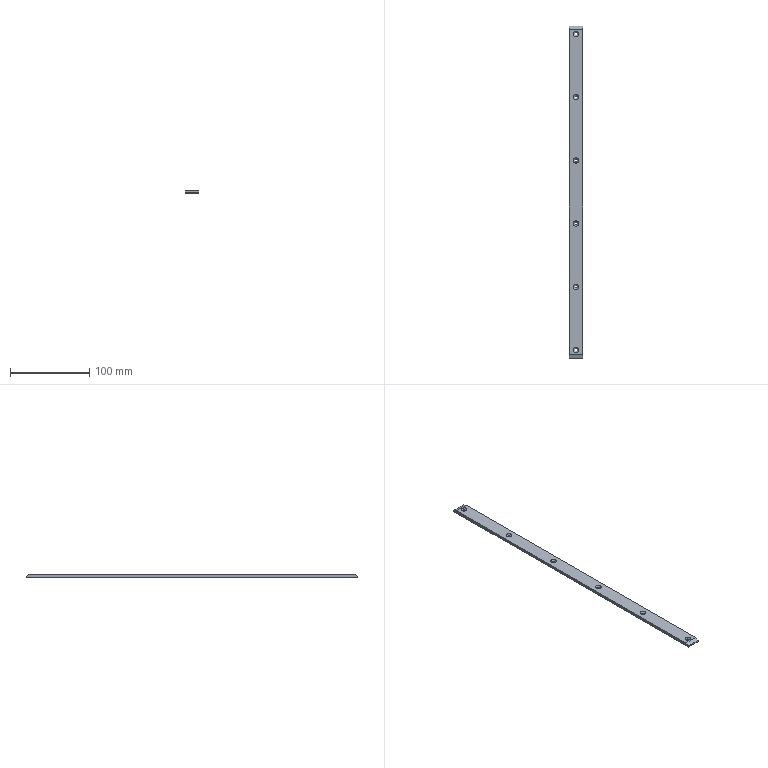Part | NX | features BREP 1 | 1 solid | 32 faces | box 17 x 420 x 4 mm | volume 28032 mm3 | cone 12 | cylinder 12 | plane 8 | commonest cylinder face diameters 3.4 x12
STEP:
#1=CARTESIAN_POINT('',(-8.5,-210.,2.));
#2=VERTEX_POINT('',#1);
#3=CARTESIAN_POINT('',(-8.5,-205.,4.));
#4=VERTEX_POINT('',#3);
#5=CARTESIAN_POINT('',(-8.5,-205.,4.));
#6=DIRECTION('',(0.,0.9285,0.3714));
#7=VECTOR('',#6,1000.);
#8=LINE('',#5,#7);
#9=EDGE_CURVE('',#2,#4,#8,.T.);
#10=ORIENTED_EDGE('',*,*,#9,.F.);
#11=CARTESIAN_POINT('',(8.5,-210.,2.));
#12=VERTEX_POINT('',#11);
#13=CARTESIAN_POINT('',(-8.5,-210.,2.));
#14=DIRECTION('',(-1.,0.,0.));
#15=VECTOR('',#14,1000.);
#16=LINE('',#13,#15);
#17=EDGE_CURVE('',#12,#2,#16,.T.);
#18=ORIENTED_EDGE('',*,*,#17,.F.);
#19=CARTESIAN_POINT('',(8.5,-205.,4.));
#20=VERTEX_POINT('',#19);
#21=CARTESIAN_POINT('',(8.5,-205.,4.));
#22=DIRECTION('',(0.,-0.9285,-0.3714));
#23=VECTOR('',#22,1000.);
#24=LINE('',#21,#23);
#25=EDGE_CURVE('',#20,#12,#24,.T.);
#26=ORIENTED_EDGE('',*,*,#25,.F.);
#27=CARTESIAN_POINT('',(0.,-205.,4.));
#28=DIRECTION('',(1.,0.,0.));
#29=VECTOR('',#28,1000.);
#30=LINE('',#27,#29);
#31=EDGE_CURVE('',#4,#20,#30,.T.);
#32=ORIENTED_EDGE('',*,*,#31,.F.);
#33=EDGE_LOOP('',(#10,#18,#26,#32));
#34=FACE_BOUND('',#33,.T.);
#35=CARTESIAN_POINT('',(0.,-205.,4.));
#36=DIRECTION('',(0.,0.3714,-0.9285));
#37=DIRECTION('',(1.,0.,0.));
#38=AXIS2_PLACEMENT_3D('',#35,#36,#37);
#39=PLANE('',#38);
#40=ADVANCED_FACE('',(#34),#39,.F.);
#41=CARTESIAN_POINT('',(8.5,210.,2.));
#42=VERTEX_POINT('',#41);
#43=CARTESIAN_POINT('',(8.5,205.,4.));
#44=VERTEX_POINT('',#43);
#45=CARTESIAN_POINT('',(8.5,205.,4.));
#46=DIRECTION('',(0.,-0.9285,0.3714));
#47=VECTOR('',#46,1000.);
#48=LINE('',#45,#47);
#49=EDGE_CURVE('',#42,#44,#48,.T.);
#50=ORIENTED_EDGE('',*,*,#49,.F.);
#51=CARTESIAN_POINT('',(-8.5,210.,2.));
#52=VERTEX_POINT('',#51);
#53=CARTESIAN_POINT('',(-8.5,210.,2.));
#54=DIRECTION('',(1.,0.,0.));
#55=VECTOR('',#54,1000.);
#56=LINE('',#53,#55);
#57=EDGE_CURVE('',#52,#42,#56,.T.);
#58=ORIENTED_EDGE('',*,*,#57,.F.);
#59=CARTESIAN_POINT('',(-8.5,205.,4.));
#60=VERTEX_POINT('',#59);
#61=CARTESIAN_POINT('',(-8.5,205.,4.));
#62=DIRECTION('',(0.,0.9285,-0.3714));
#63=VECTOR('',#62,1000.);
#64=LINE('',#61,#63);
#65=EDGE_CURVE('',#60,#52,#64,.T.);
#66=ORIENTED_EDGE('',*,*,#65,.F.);
#67=CARTESIAN_POINT('',(0.,205.,4.));
#68=DIRECTION('',(-1.,0.,0.));
#69=VECTOR('',#68,1000.);
#70=LINE('',#67,#69);
#71=EDGE_CURVE('',#44,#60,#70,.T.);
#72=ORIENTED_EDGE('',*,*,#71,.F.);
#73=EDGE_LOOP('',(#50,#58,#66,#72));
#74=FACE_BOUND('',#73,.T.);
#75=CARTESIAN_POINT('',(0.,205.,4.));
#76=DIRECTION('',(0.,-0.3714,-0.9285));
#77=DIRECTION('',(-1.,0.,0.));
#78=AXIS2_PLACEMENT_3D('',#75,#76,#77);
#79=PLANE('',#78);
#80=ADVANCED_FACE('',(#74),#79,.F.);
#81=CARTESIAN_POINT('',(-3.5,-200.,4.));
#82=VERTEX_POINT('',#81);
#83=CARTESIAN_POINT('',(-1.7,-200.,2.2));
#84=VERTEX_POINT('',#83);
#85=CARTESIAN_POINT('',(-3.5,-200.,4.));
#86=DIRECTION('',(-0.7071,0.,0.7071));
#87=VECTOR('',#86,1000.);
#88=LINE('',#85,#87);
#89=EDGE_CURVE('',#82,#84,#88,.F.);
#90=ORIENTED_EDGE('',*,*,#89,.T.);
#91=CARTESIAN_POINT('',(1.7,-200.,2.2));
#92=VERTEX_POINT('',#91);
#93=CARTESIAN_POINT('',(0.,-200.,2.2));
#94=DIRECTION('',(0.,0.,1.));
#95=DIRECTION('',(1.,0.,0.));
#96=AXIS2_PLACEMENT_3D('',#93,#94,#95);
#97=CIRCLE('',#96,1.7);
#98=EDGE_CURVE('',#92,#84,#97,.T.);
#99=ORIENTED_EDGE('',*,*,#98,.F.);
#100=CARTESIAN_POINT('',(3.5,-200.,4.));
#101=VERTEX_POINT('',#100);
#102=CARTESIAN_POINT('',(3.5,-200.,4.));
#103=DIRECTION('',(0.7071,0.,0.7071));
#104=VECTOR('',#103,1000.);
#105=LINE('',#102,#104);
#106=EDGE_CURVE('',#101,#92,#105,.F.);
#107=ORIENTED_EDGE('',*,*,#106,.F.);
#108=CARTESIAN_POINT('',(0.,-200.,4.));
#109=DIRECTION('',(0.,0.,1.));
#110=DIRECTION('',(1.,0.,0.));
#111=AXIS2_PLACEMENT_3D('',#108,#109,#110);
#112=CIRCLE('',#111,3.5);
#113=EDGE_CURVE('',#101,#82,#112,.T.);
#114=ORIENTED_EDGE('',*,*,#113,.T.);
#115=EDGE_LOOP('',(#90,#99,#107,#114));
#116=FACE_BOUND('',#115,.T.);
#117=CARTESIAN_POINT('',(0.,-200.,4.));
#118=DIRECTION('',(0.,0.,1.));
#119=DIRECTION('',(1.,0.,0.));
#120=AXIS2_PLACEMENT_3D('',#117,#118,#119);
#121=CONICAL_SURFACE('',#120,3.5,0.7854);
#122=ADVANCED_FACE('',(#116),#121,.F.);
#123=CARTESIAN_POINT('',(-1.7,-200.,0.));
#124=VERTEX_POINT('',#123);
#125=CARTESIAN_POINT('',(-1.7,-200.,4.));
#126=DIRECTION('',(0.,0.,1.));
#127=VECTOR('',#126,1000.);
#128=LINE('',#125,#127);
#129=EDGE_CURVE('',#84,#124,#128,.F.);
#130=ORIENTED_EDGE('',*,*,#129,.T.);
#131=CARTESIAN_POINT('',(1.7,-200.,0.));
#132=VERTEX_POINT('',#131);
#133=CARTESIAN_POINT('',(0.,-200.,0.));
#134=DIRECTION('',(0.,0.,-1.));
#135=DIRECTION('',(-1.,0.,0.));
#136=AXIS2_PLACEMENT_3D('',#133,#134,#135);
#137=CIRCLE('',#136,1.7);
#138=EDGE_CURVE('',#124,#132,#137,.T.);
#139=ORIENTED_EDGE('',*,*,#138,.T.);
#140=CARTESIAN_POINT('',(1.7,-200.,4.));
#141=DIRECTION('',(0.,0.,1.));
#142=VECTOR('',#141,1000.);
#143=LINE('',#140,#142);
#144=EDGE_CURVE('',#92,#132,#143,.F.);
#145=ORIENTED_EDGE('',*,*,#144,.F.);
#146=ORIENTED_EDGE('',*,*,#98,.T.);
#147=EDGE_LOOP('',(#130,#139,#145,#146));
#148=FACE_BOUND('',#147,.T.);
#149=CARTESIAN_POINT('',(0.,-200.,4.));
#150=DIRECTION('',(0.,0.,1.));
#151=DIRECTION('',(1.,0.,0.));
#152=AXIS2_PLACEMENT_3D('',#149,#150,#151);
#153=CYLINDRICAL_SURFACE('',#152,1.7);
#154=ADVANCED_FACE('',(#148),#153,.F.);
#155=CARTESIAN_POINT('',(-3.5,-120.,4.));
#156=VERTEX_POINT('',#155);
#157=CARTESIAN_POINT('',(-1.7,-120.,2.2));
#158=VERTEX_POINT('',#157);
#159=CARTESIAN_POINT('',(-3.5,-120.,4.));
#160=DIRECTION('',(-0.7071,0.,0.7071));
#161=VECTOR('',#160,1000.);
#162=LINE('',#159,#161);
#163=EDGE_CURVE('',#156,#158,#162,.F.);
#164=ORIENTED_EDGE('',*,*,#163,.T.);
#165=CARTESIAN_POINT('',(1.7,-120.,2.2));
#166=VERTEX_POINT('',#165);
#167=CARTESIAN_POINT('',(0.,-120.,2.2));
#168=DIRECTION('',(0.,0.,1.));
#169=DIRECTION('',(1.,0.,0.));
#170=AXIS2_PLACEMENT_3D('',#167,#168,#169);
#171=CIRCLE('',#170,1.7);
#172=EDGE_CURVE('',#166,#158,#171,.T.);
#173=ORIENTED_EDGE('',*,*,#172,.F.);
#174=CARTESIAN_POINT('',(3.5,-120.,4.));
#175=VERTEX_POINT('',#174);
#176=CARTESIAN_POINT('',(3.5,-120.,4.));
#177=DIRECTION('',(0.7071,0.,0.7071));
#178=VECTOR('',#177,1000.);
#179=LINE('',#176,#178);
#180=EDGE_CURVE('',#175,#166,#179,.F.);
#181=ORIENTED_EDGE('',*,*,#180,.F.);
#182=CARTESIAN_POINT('',(0.,-120.,4.));
#183=DIRECTION('',(0.,0.,1.));
#184=DIRECTION('',(1.,0.,0.));
#185=AXIS2_PLACEMENT_3D('',#182,#183,#184);
#186=CIRCLE('',#185,3.5);
#187=EDGE_CURVE('',#175,#156,#186,.T.);
#188=ORIENTED_EDGE('',*,*,#187,.T.);
#189=EDGE_LOOP('',(#164,#173,#181,#188));
#190=FACE_BOUND('',#189,.T.);
#191=CARTESIAN_POINT('',(0.,-120.,4.));
#192=DIRECTION('',(0.,0.,1.));
#193=DIRECTION('',(1.,0.,0.));
#194=AXIS2_PLACEMENT_3D('',#191,#192,#193);
#195=CONICAL_SURFACE('',#194,3.5,0.7854);
#196=ADVANCED_FACE('',(#190),#195,.F.);
#197=CARTESIAN_POINT('',(-1.7,-120.,0.));
#198=VERTEX_POINT('',#197);
#199=CARTESIAN_POINT('',(-1.7,-120.,4.));
#200=DIRECTION('',(0.,0.,1.));
#201=VECTOR('',#200,1000.);
#202=LINE('',#199,#201);
#203=EDGE_CURVE('',#158,#198,#202,.F.);
#204=ORIENTED_EDGE('',*,*,#203,.T.);
#205=CARTESIAN_POINT('',(1.7,-120.,0.));
#206=VERTEX_POINT('',#205);
#207=CARTESIAN_POINT('',(0.,-120.,0.));
#208=DIRECTION('',(0.,0.,-1.));
#209=DIRECTION('',(-1.,0.,0.));
#210=AXIS2_PLACEMENT_3D('',#207,#208,#209);
#211=CIRCLE('',#210,1.7);
#212=EDGE_CURVE('',#198,#206,#211,.T.);
#213=ORIENTED_EDGE('',*,*,#212,.T.);
#214=CARTESIAN_POINT('',(1.7,-120.,4.));
#215=DIRECTION('',(0.,0.,1.));
#216=VECTOR('',#215,1000.);
#217=LINE('',#214,#216);
#218=EDGE_CURVE('',#166,#206,#217,.F.);
#219=ORIENTED_EDGE('',*,*,#218,.F.);
#220=ORIENTED_EDGE('',*,*,#172,.T.);
#221=EDGE_LOOP('',(#204,#213,#219,#220));
#222=FACE_BOUND('',#221,.T.);
#223=CARTESIAN_POINT('',(0.,-120.,4.));
#224=DIRECTION('',(0.,0.,1.));
#225=DIRECTION('',(1.,0.,0.));
#226=AXIS2_PLACEMENT_3D('',#223,#224,#225);
#227=CYLINDRICAL_SURFACE('',#226,1.7);
#228=ADVANCED_FACE('',(#222),#227,.F.);
#229=CARTESIAN_POINT('',(-3.5,-40.,4.));
#230=VERTEX_POINT('',#229);
#231=CARTESIAN_POINT('',(-1.7,-40.,2.2));
#232=VERTEX_POINT('',#231);
#233=CARTESIAN_POINT('',(-3.5,-40.,4.));
#234=DIRECTION('',(-0.7071,0.,0.7071));
#235=VECTOR('',#234,1000.);
#236=LINE('',#233,#235);
#237=EDGE_CURVE('',#230,#232,#236,.F.);
#238=ORIENTED_EDGE('',*,*,#237,.T.);
#239=CARTESIAN_POINT('',(1.7,-40.,2.2));
#240=VERTEX_POINT('',#239);
#241=CARTESIAN_POINT('',(0.,-40.,2.2));
#242=DIRECTION('',(0.,0.,1.));
#243=DIRECTION('',(1.,0.,0.));
#244=AXIS2_PLACEMENT_3D('',#241,#242,#243);
#245=CIRCLE('',#244,1.7);
#246=EDGE_CURVE('',#240,#232,#245,.T.);
#247=ORIENTED_EDGE('',*,*,#246,.F.);
#248=CARTESIAN_POINT('',(3.5,-40.,4.));
#249=VERTEX_POINT('',#248);
#250=CARTESIAN_POINT('',(3.5,-40.,4.));
#251=DIRECTION('',(0.7071,0.,0.7071));
#252=VECTOR('',#251,1000.);
#253=LINE('',#250,#252);
#254=EDGE_CURVE('',#249,#240,#253,.F.);
#255=ORIENTED_EDGE('',*,*,#254,.F.);
#256=CARTESIAN_POINT('',(0.,-40.,4.));
#257=DIRECTION('',(0.,0.,1.));
#258=DIRECTION('',(1.,0.,0.));
#259=AXIS2_PLACEMENT_3D('',#256,#257,#258);
#260=CIRCLE('',#259,3.5);
#261=EDGE_CURVE('',#249,#230,#260,.T.);
#262=ORIENTED_EDGE('',*,*,#261,.T.);
#263=EDGE_LOOP('',(#238,#247,#255,#262));
#264=FACE_BOUND('',#263,.T.);
#265=CARTESIAN_POINT('',(0.,-40.,4.));
#266=DIRECTION('',(0.,0.,1.));
#267=DIRECTION('',(1.,0.,0.));
#268=AXIS2_PLACEMENT_3D('',#265,#266,#267);
#269=CONICAL_SURFACE('',#268,3.5,0.7854);
#270=ADVANCED_FACE('',(#264),#269,.F.);
#271=CARTESIAN_POINT('',(-1.7,-40.,0.));
#272=VERTEX_POINT('',#271);
#273=CARTESIAN_POINT('',(-1.7,-40.,4.));
#274=DIRECTION('',(0.,0.,1.));
#275=VECTOR('',#274,1000.);
#276=LINE('',#273,#275);
#277=EDGE_CURVE('',#232,#272,#276,.F.);
#278=ORIENTED_EDGE('',*,*,#277,.T.);
#279=CARTESIAN_POINT('',(1.7,-40.,0.));
#280=VERTEX_POINT('',#279);
#281=CARTESIAN_POINT('',(0.,-40.,0.));
#282=DIRECTION('',(0.,0.,-1.));
#283=DIRECTION('',(-1.,0.,0.));
#284=AXIS2_PLACEMENT_3D('',#281,#282,#283);
#285=CIRCLE('',#284,1.7);
#286=EDGE_CURVE('',#272,#280,#285,.T.);
#287=ORIENTED_EDGE('',*,*,#286,.T.);
#288=CARTESIAN_POINT('',(1.7,-40.,4.));
#289=DIRECTION('',(0.,0.,1.));
#290=VECTOR('',#289,1000.);
#291=LINE('',#288,#290);
#292=EDGE_CURVE('',#240,#280,#291,.F.);
#293=ORIENTED_EDGE('',*,*,#292,.F.);
#294=ORIENTED_EDGE('',*,*,#246,.T.);
#295=EDGE_LOOP('',(#278,#287,#293,#294));
#296=FACE_BOUND('',#295,.T.);
#297=CARTESIAN_POINT('',(0.,-40.,4.));
#298=DIRECTION('',(0.,0.,1.));
#299=DIRECTION('',(1.,0.,0.));
#300=AXIS2_PLACEMENT_3D('',#297,#298,#299);
#301=CYLINDRICAL_SURFACE('',#300,1.7);
#302=ADVANCED_FACE('',(#296),#301,.F.);
#303=CARTESIAN_POINT('',(-3.5,40.,4.));
#304=VERTEX_POINT('',#303);
#305=CARTESIAN_POINT('',(-1.7,40.,2.2));
#306=VERTEX_POINT('',#305);
#307=CARTESIAN_POINT('',(-3.5,40.,4.));
#308=DIRECTION('',(-0.7071,0.,0.7071));
#309=VECTOR('',#308,1000.);
#310=LINE('',#307,#309);
#311=EDGE_CURVE('',#304,#306,#310,.F.);
#312=ORIENTED_EDGE('',*,*,#311,.T.);
#313=CARTESIAN_POINT('',(1.7,40.,2.2));
#314=VERTEX_POINT('',#313);
#315=CARTESIAN_POINT('',(0.,40.,2.2));
#316=DIRECTION('',(0.,0.,1.));
#317=DIRECTION('',(1.,0.,0.));
#318=AXIS2_PLACEMENT_3D('',#315,#316,#317);
#319=CIRCLE('',#318,1.7);
#320=EDGE_CURVE('',#314,#306,#319,.T.);
#321=ORIENTED_EDGE('',*,*,#320,.F.);
#322=CARTESIAN_POINT('',(3.5,40.,4.));
#323=VERTEX_POINT('',#322);
#324=CARTESIAN_POINT('',(3.5,40.,4.));
#325=DIRECTION('',(0.7071,0.,0.7071));
#326=VECTOR('',#325,1000.);
#327=LINE('',#324,#326);
#328=EDGE_CURVE('',#323,#314,#327,.F.);
#329=ORIENTED_EDGE('',*,*,#328,.F.);
#330=CARTESIAN_POINT('',(0.,40.,4.));
#331=DIRECTION('',(0.,0.,1.));
#332=DIRECTION('',(1.,0.,0.));
#333=AXIS2_PLACEMENT_3D('',#330,#331,#332);
#334=CIRCLE('',#333,3.5);
#335=EDGE_CURVE('',#323,#304,#334,.T.);
#336=ORIENTED_EDGE('',*,*,#335,.T.);
#337=EDGE_LOOP('',(#312,#321,#329,#336));
#338=FACE_BOUND('',#337,.T.);
#339=CARTESIAN_POINT('',(0.,40.,4.));
#340=DIRECTION('',(0.,0.,1.));
#341=DIRECTION('',(1.,0.,0.));
#342=AXIS2_PLACEMENT_3D('',#339,#340,#341);
#343=CONICAL_SURFACE('',#342,3.5,0.7854);
#344=ADVANCED_FACE('',(#338),#343,.F.);
#345=CARTESIAN_POINT('',(-1.7,40.,0.));
#346=VERTEX_POINT('',#345);
#347=CARTESIAN_POINT('',(-1.7,40.,4.));
#348=DIRECTION('',(0.,0.,1.));
#349=VECTOR('',#348,1000.);
#350=LINE('',#347,#349);
#351=EDGE_CURVE('',#306,#346,#350,.F.);
#352=ORIENTED_EDGE('',*,*,#351,.T.);
#353=CARTESIAN_POINT('',(1.7,40.,0.));
#354=VERTEX_POINT('',#353);
#355=CARTESIAN_POINT('',(0.,40.,0.));
#356=DIRECTION('',(0.,0.,-1.));
#357=DIRECTION('',(-1.,0.,0.));
#358=AXIS2_PLACEMENT_3D('',#355,#356,#357);
#359=CIRCLE('',#358,1.7);
#360=EDGE_CURVE('',#346,#354,#359,.T.);
#361=ORIENTED_EDGE('',*,*,#360,.T.);
#362=CARTESIAN_POINT('',(1.7,40.,4.));
#363=DIRECTION('',(0.,0.,1.));
#364=VECTOR('',#363,1000.);
#365=LINE('',#362,#364);
#366=EDGE_CURVE('',#314,#354,#365,.F.);
#367=ORIENTED_EDGE('',*,*,#366,.F.);
#368=ORIENTED_EDGE('',*,*,#320,.T.);
#369=EDGE_LOOP('',(#352,#361,#367,#368));
#370=FACE_BOUND('',#369,.T.);
#371=CARTESIAN_POINT('',(0.,40.,4.));
#372=DIRECTION('',(0.,0.,1.));
#373=DIRECTION('',(1.,0.,0.));
#374=AXIS2_PLACEMENT_3D('',#371,#372,#373);
#375=CYLINDRICAL_SURFACE('',#374,1.7);
#376=ADVANCED_FACE('',(#370),#375,.F.);
#377=CARTESIAN_POINT('',(-3.5,120.,4.));
#378=VERTEX_POINT('',#377);
#379=CARTESIAN_POINT('',(-1.7,120.,2.2));
#380=VERTEX_POINT('',#379);
#381=CARTESIAN_POINT('',(-3.5,120.,4.));
#382=DIRECTION('',(-0.7071,0.,0.7071));
#383=VECTOR('',#382,1000.);
#384=LINE('',#381,#383);
#385=EDGE_CURVE('',#378,#380,#384,.F.);
#386=ORIENTED_EDGE('',*,*,#385,.T.);
#387=CARTESIAN_POINT('',(1.7,120.,2.2));
#388=VERTEX_POINT('',#387);
#389=CARTESIAN_POINT('',(0.,120.,2.2));
#390=DIRECTION('',(0.,0.,1.));
#391=DIRECTION('',(1.,0.,0.));
#392=AXIS2_PLACEMENT_3D('',#389,#390,#391);
#393=CIRCLE('',#392,1.7);
#394=EDGE_CURVE('',#388,#380,#393,.T.);
#395=ORIENTED_EDGE('',*,*,#394,.F.);
#396=CARTESIAN_POINT('',(3.5,120.,4.));
#397=VERTEX_POINT('',#396);
#398=CARTESIAN_POINT('',(3.5,120.,4.));
#399=DIRECTION('',(0.7071,0.,0.7071));
#400=VECTOR('',#399,1000.);
#401=LINE('',#398,#400);
#402=EDGE_CURVE('',#397,#388,#401,.F.);
#403=ORIENTED_EDGE('',*,*,#402,.F.);
#404=CARTESIAN_POINT('',(0.,120.,4.));
#405=DIRECTION('',(0.,0.,1.));
#406=DIRECTION('',(1.,0.,0.));
#407=AXIS2_PLACEMENT_3D('',#404,#405,#406);
#408=CIRCLE('',#407,3.5);
#409=EDGE_CURVE('',#397,#378,#408,.T.);
#410=ORIENTED_EDGE('',*,*,#409,.T.);
#411=EDGE_LOOP('',(#386,#395,#403,#410));
#412=FACE_BOUND('',#411,.T.);
#413=CARTESIAN_POINT('',(0.,120.,4.));
#414=DIRECTION('',(0.,0.,1.));
#415=DIRECTION('',(1.,0.,0.));
#416=AXIS2_PLACEMENT_3D('',#413,#414,#415);
#417=CONICAL_SURFACE('',#416,3.5,0.7854);
#418=ADVANCED_FACE('',(#412),#417,.F.);
#419=CARTESIAN_POINT('',(-1.7,120.,0.));
#420=VERTEX_POINT('',#419);
#421=CARTESIAN_POINT('',(-1.7,120.,4.));
#422=DIRECTION('',(0.,0.,1.));
#423=VECTOR('',#422,1000.);
#424=LINE('',#421,#423);
#425=EDGE_CURVE('',#380,#420,#424,.F.);
#426=ORIENTED_EDGE('',*,*,#425,.T.);
#427=CARTESIAN_POINT('',(1.7,120.,0.));
#428=VERTEX_POINT('',#427);
#429=CARTESIAN_POINT('',(0.,120.,0.));
#430=DIRECTION('',(0.,0.,-1.));
#431=DIRECTION('',(-1.,0.,0.));
#432=AXIS2_PLACEMENT_3D('',#429,#430,#431);
#433=CIRCLE('',#432,1.7);
#434=EDGE_CURVE('',#420,#428,#433,.T.);
#435=ORIENTED_EDGE('',*,*,#434,.T.);
#436=CARTESIAN_POINT('',(1.7,120.,4.));
#437=DIRECTION('',(0.,0.,1.));
#438=VECTOR('',#437,1000.);
#439=LINE('',#436,#438);
#440=EDGE_CURVE('',#388,#428,#439,.F.);
#441=ORIENTED_EDGE('',*,*,#440,.F.);
#442=ORIENTED_EDGE('',*,*,#394,.T.);
#443=EDGE_LOOP('',(#426,#435,#441,#442));
#444=FACE_BOUND('',#443,.T.);
#445=CARTESIAN_POINT('',(0.,120.,4.));
#446=DIRECTION('',(0.,0.,1.));
#447=DIRECTION('',(1.,0.,0.));
#448=AXIS2_PLACEMENT_3D('',#445,#446,#447);
#449=CYLINDRICAL_SURFACE('',#448,1.7);
#450=ADVANCED_FACE('',(#444),#449,.F.);
#451=CARTESIAN_POINT('',(-3.5,200.,4.));
#452=VERTEX_POINT('',#451);
#453=CARTESIAN_POINT('',(-1.7,200.,2.2));
#454=VERTEX_POINT('',#453);
#455=CARTESIAN_POINT('',(-3.5,200.,4.));
#456=DIRECTION('',(-0.7071,0.,0.7071));
#457=VECTOR('',#456,1000.);
#458=LINE('',#455,#457);
#459=EDGE_CURVE('',#452,#454,#458,.F.);
#460=ORIENTED_EDGE('',*,*,#459,.T.);
#461=CARTESIAN_POINT('',(1.7,200.,2.2));
#462=VERTEX_POINT('',#461);
#463=CARTESIAN_POINT('',(0.,200.,2.2));
#464=DIRECTION('',(0.,0.,1.));
#465=DIRECTION('',(1.,0.,0.));
#466=AXIS2_PLACEMENT_3D('',#463,#464,#465);
#467=CIRCLE('',#466,1.7);
#468=EDGE_CURVE('',#462,#454,#467,.T.);
#469=ORIENTED_EDGE('',*,*,#468,.F.);
#470=CARTESIAN_POINT('',(3.5,200.,4.));
#471=VERTEX_POINT('',#470);
#472=CARTESIAN_POINT('',(3.5,200.,4.));
#473=DIRECTION('',(0.7071,0.,0.7071));
#474=VECTOR('',#473,1000.);
#475=LINE('',#472,#474);
#476=EDGE_CURVE('',#471,#462,#475,.F.);
#477=ORIENTED_EDGE('',*,*,#476,.F.);
#478=CARTESIAN_POINT('',(0.,200.,4.));
#479=DIRECTION('',(0.,0.,1.));
#480=DIRECTION('',(1.,0.,0.));
#481=AXIS2_PLACEMENT_3D('',#478,#479,#480);
#482=CIRCLE('',#481,3.5);
#483=EDGE_CURVE('',#471,#452,#482,.T.);
#484=ORIENTED_EDGE('',*,*,#483,.T.);
#485=EDGE_LOOP('',(#460,#469,#477,#484));
#486=FACE_BOUND('',#485,.T.);
#487=CARTESIAN_POINT('',(0.,200.,4.));
#488=DIRECTION('',(0.,0.,1.));
#489=DIRECTION('',(1.,0.,0.));
#490=AXIS2_PLACEMENT_3D('',#487,#488,#489);
#491=CONICAL_SURFACE('',#490,3.5,0.7854);
#492=ADVANCED_FACE('',(#486),#491,.F.);
#493=CARTESIAN_POINT('',(-1.7,200.,0.));
#494=VERTEX_POINT('',#493);
#495=CARTESIAN_POINT('',(-1.7,200.,4.));
#496=DIRECTION('',(0.,0.,1.));
#497=VECTOR('',#496,1000.);
#498=LINE('',#495,#497);
#499=EDGE_CURVE('',#454,#494,#498,.F.);
#500=ORIENTED_EDGE('',*,*,#499,.T.);
#501=CARTESIAN_POINT('',(1.7,200.,0.));
#502=VERTEX_POINT('',#501);
#503=CARTESIAN_POINT('',(0.,200.,0.));
#504=DIRECTION('',(0.,0.,-1.));
#505=DIRECTION('',(-1.,0.,0.));
#506=AXIS2_PLACEMENT_3D('',#503,#504,#505);
#507=CIRCLE('',#506,1.7);
#508=EDGE_CURVE('',#494,#502,#507,.T.);
#509=ORIENTED_EDGE('',*,*,#508,.T.);
#510=CARTESIAN_POINT('',(1.7,200.,4.));
#511=DIRECTION('',(0.,0.,1.));
#512=VECTOR('',#511,1000.);
#513=LINE('',#510,#512);
#514=EDGE_CURVE('',#462,#502,#513,.F.);
#515=ORIENTED_EDGE('',*,*,#514,.F.);
#516=ORIENTED_EDGE('',*,*,#468,.T.);
#517=EDGE_LOOP('',(#500,#509,#515,#516));
#518=FACE_BOUND('',#517,.T.);
#519=CARTESIAN_POINT('',(0.,200.,4.));
#520=DIRECTION('',(0.,0.,1.));
#521=DIRECTION('',(1.,0.,0.));
#522=AXIS2_PLACEMENT_3D('',#519,#520,#521);
#523=CYLINDRICAL_SURFACE('',#522,1.7);
#524=ADVANCED_FACE('',(#518),#523,.F.);
#525=CARTESIAN_POINT('',(8.5,-210.,0.));
#526=VERTEX_POINT('',#525);
#527=CARTESIAN_POINT('',(8.5,210.,0.));
#528=VERTEX_POINT('',#527);
#529=CARTESIAN_POINT('',(8.5,-210.,0.));
#530=DIRECTION('',(0.,1.,0.));
#531=VECTOR('',#530,1000.);
#532=LINE('',#529,#531);
#533=EDGE_CURVE('',#526,#528,#532,.T.);
#534=ORIENTED_EDGE('',*,*,#533,.F.);
#535=CARTESIAN_POINT('',(-8.5,-210.,0.));
#536=VERTEX_POINT('',#535);
#537=CARTESIAN_POINT('',(-8.5,-210.,0.));
#538=DIRECTION('',(1.,0.,0.));
#539=VECTOR('',#538,1000.);
#540=LINE('',#537,#539);
#541=EDGE_CURVE('',#536,#526,#540,.T.);
#542=ORIENTED_EDGE('',*,*,#541,.F.);
#543=CARTESIAN_POINT('',(-8.5,210.,0.));
#544=VERTEX_POINT('',#543);
#545=CARTESIAN_POINT('',(-8.5,-210.,0.));
#546=DIRECTION('',(0.,-1.,0.));
#547=VECTOR('',#546,1000.);
#548=LINE('',#545,#547);
#549=EDGE_CURVE('',#544,#536,#548,.T.);
#550=ORIENTED_EDGE('',*,*,#549,.F.);
#551=CARTESIAN_POINT('',(-8.5,210.,0.));
#552=DIRECTION('',(-1.,0.,0.));
#553=VECTOR('',#552,1000.);
#554=LINE('',#551,#553);
#555=EDGE_CURVE('',#528,#544,#554,.T.);
#556=ORIENTED_EDGE('',*,*,#555,.F.);
#557=EDGE_LOOP('',(#534,#542,#550,#556));
#558=FACE_BOUND('',#557,.T.);
#559=CARTESIAN_POINT('',(0.,200.,0.));
#560=DIRECTION('',(0.,0.,-1.));
#561=DIRECTION('',(-1.,0.,0.));
#562=AXIS2_PLACEMENT_3D('',#559,#560,#561);
#563=CIRCLE('',#562,1.7);
#564=EDGE_CURVE('',#502,#494,#563,.T.);
#565=ORIENTED_EDGE('',*,*,#564,.F.);
#566=ORIENTED_EDGE('',*,*,#508,.F.);
#567=EDGE_LOOP('',(#565,#566));
#568=FACE_BOUND('',#567,.T.);
#569=CARTESIAN_POINT('',(0.,120.,0.));
#570=DIRECTION('',(0.,0.,-1.));
#571=DIRECTION('',(-1.,0.,0.));
#572=AXIS2_PLACEMENT_3D('',#569,#570,#571);
#573=CIRCLE('',#572,1.7);
#574=EDGE_CURVE('',#428,#420,#573,.T.);
#575=ORIENTED_EDGE('',*,*,#574,.F.);
#576=ORIENTED_EDGE('',*,*,#434,.F.);
#577=EDGE_LOOP('',(#575,#576));
#578=FACE_BOUND('',#577,.T.);
#579=CARTESIAN_POINT('',(0.,40.,0.));
#580=DIRECTION('',(0.,0.,-1.));
#581=DIRECTION('',(-1.,0.,0.));
#582=AXIS2_PLACEMENT_3D('',#579,#580,#581);
#583=CIRCLE('',#582,1.7);
#584=EDGE_CURVE('',#354,#346,#583,.T.);
#585=ORIENTED_EDGE('',*,*,#584,.F.);
#586=ORIENTED_EDGE('',*,*,#360,.F.);
#587=EDGE_LOOP('',(#585,#586));
#588=FACE_BOUND('',#587,.T.);
#589=CARTESIAN_POINT('',(0.,-40.,0.));
#590=DIRECTION('',(0.,0.,-1.));
#591=DIRECTION('',(-1.,0.,0.));
#592=AXIS2_PLACEMENT_3D('',#589,#590,#591);
#593=CIRCLE('',#592,1.7);
#594=EDGE_CURVE('',#280,#272,#593,.T.);
#595=ORIENTED_EDGE('',*,*,#594,.F.);
#596=ORIENTED_EDGE('',*,*,#286,.F.);
#597=EDGE_LOOP('',(#595,#596));
#598=FACE_BOUND('',#597,.T.);
#599=CARTESIAN_POINT('',(0.,-120.,0.));
#600=DIRECTION('',(0.,0.,-1.));
#601=DIRECTION('',(-1.,0.,0.));
#602=AXIS2_PLACEMENT_3D('',#599,#600,#601);
#603=CIRCLE('',#602,1.7);
#604=EDGE_CURVE('',#206,#198,#603,.T.);
#605=ORIENTED_EDGE('',*,*,#604,.F.);
#606=ORIENTED_EDGE('',*,*,#212,.F.);
#607=EDGE_LOOP('',(#605,#606));
#608=FACE_BOUND('',#607,.T.);
#609=CARTESIAN_POINT('',(0.,-200.,0.));
#610=DIRECTION('',(0.,0.,-1.));
#611=DIRECTION('',(-1.,0.,0.));
#612=AXIS2_PLACEMENT_3D('',#609,#610,#611);
#613=CIRCLE('',#612,1.7);
#614=EDGE_CURVE('',#132,#124,#613,.T.);
#615=ORIENTED_EDGE('',*,*,#614,.F.);
#616=ORIENTED_EDGE('',*,*,#138,.F.);
#617=EDGE_LOOP('',(#615,#616));
#618=FACE_BOUND('',#617,.T.);
#619=CARTESIAN_POINT('',(0.,0.,0.));
#620=DIRECTION('',(0.,0.,-1.));
#621=DIRECTION('',(-1.,0.,0.));
#622=AXIS2_PLACEMENT_3D('',#619,#620,#621);
#623=PLANE('',#622);
#624=ADVANCED_FACE('',(#558,#568,#578,#588,#598,#608,#618),#623,.T.);
#625=CARTESIAN_POINT('',(8.5,-210.,4.));
#626=DIRECTION('',(0.,0.,-1.));
#627=VECTOR('',#626,1000.);
#628=LINE('',#625,#627);
#629=EDGE_CURVE('',#12,#526,#628,.T.);
#630=ORIENTED_EDGE('',*,*,#629,.F.);
#631=ORIENTED_EDGE('',*,*,#17,.T.);
#632=CARTESIAN_POINT('',(-8.5,-210.,4.));
#633=DIRECTION('',(0.,0.,-1.));
#634=VECTOR('',#633,1000.);
#635=LINE('',#632,#634);
#636=EDGE_CURVE('',#2,#536,#635,.T.);
#637=ORIENTED_EDGE('',*,*,#636,.T.);
#638=ORIENTED_EDGE('',*,*,#541,.T.);
#639=EDGE_LOOP('',(#630,#631,#637,#638));
#640=FACE_BOUND('',#639,.T.);
#641=CARTESIAN_POINT('',(-8.5,-210.,4.));
#642=DIRECTION('',(0.,1.,0.));
#643=DIRECTION('',(0.,0.,1.));
#644=AXIS2_PLACEMENT_3D('',#641,#642,#643);
#645=PLANE('',#644);
#646=ADVANCED_FACE('',(#640),#645,.F.);
#647=ORIENTED_EDGE('',*,*,#636,.F.);
#648=ORIENTED_EDGE('',*,*,#9,.T.);
#649=CARTESIAN_POINT('',(-8.5,-210.,4.));
#650=DIRECTION('',(0.,-1.,0.));
#651=VECTOR('',#650,1000.);
#652=LINE('',#649,#651);
#653=EDGE_CURVE('',#60,#4,#652,.T.);
#654=ORIENTED_EDGE('',*,*,#653,.F.);
#655=ORIENTED_EDGE('',*,*,#65,.T.);
#656=CARTESIAN_POINT('',(-8.5,210.,4.));
#657=DIRECTION('',(0.,0.,-1.));
#658=VECTOR('',#657,1000.);
#659=LINE('',#656,#658);
#660=EDGE_CURVE('',#52,#544,#659,.T.);
#661=ORIENTED_EDGE('',*,*,#660,.T.);
#662=ORIENTED_EDGE('',*,*,#549,.T.);
#663=EDGE_LOOP('',(#647,#648,#654,#655,#661,#662));
#664=FACE_BOUND('',#663,.T.);
#665=CARTESIAN_POINT('',(-8.5,-210.,4.));
#666=DIRECTION('',(1.,0.,0.));
#667=DIRECTION('',(0.,0.,-1.));
#668=AXIS2_PLACEMENT_3D('',#665,#666,#667);
#669=PLANE('',#668);
#670=ADVANCED_FACE('',(#664),#669,.F.);
#671=ORIENTED_EDGE('',*,*,#660,.F.);
#672=ORIENTED_EDGE('',*,*,#57,.T.);
#673=CARTESIAN_POINT('',(8.5,210.,4.));
#674=DIRECTION('',(0.,0.,-1.));
#675=VECTOR('',#674,1000.);
#676=LINE('',#673,#675);
#677=EDGE_CURVE('',#42,#528,#676,.T.);
#678=ORIENTED_EDGE('',*,*,#677,.T.);
#679=ORIENTED_EDGE('',*,*,#555,.T.);
#680=EDGE_LOOP('',(#671,#672,#678,#679));
#681=FACE_BOUND('',#680,.T.);
#682=CARTESIAN_POINT('',(-8.5,210.,4.));
#683=DIRECTION('',(0.,-1.,0.));
#684=DIRECTION('',(0.,0.,-1.));
#685=AXIS2_PLACEMENT_3D('',#682,#683,#684);
#686=PLANE('',#685);
#687=ADVANCED_FACE('',(#681),#686,.F.);
#688=CARTESIAN_POINT('',(8.5,-210.,4.));
#689=DIRECTION('',(0.,1.,0.));
#690=VECTOR('',#689,1000.);
#691=LINE('',#688,#690);
#692=EDGE_CURVE('',#20,#44,#691,.T.);
#693=ORIENTED_EDGE('',*,*,#692,.F.);
#694=ORIENTED_EDGE('',*,*,#25,.T.);
#695=ORIENTED_EDGE('',*,*,#629,.T.);
#696=ORIENTED_EDGE('',*,*,#533,.T.);
#697=ORIENTED_EDGE('',*,*,#677,.F.);
#698=ORIENTED_EDGE('',*,*,#49,.T.);
#699=EDGE_LOOP('',(#693,#694,#695,#696,#697,#698));
#700=FACE_BOUND('',#699,.T.);
#701=CARTESIAN_POINT('',(8.5,-210.,4.));
#702=DIRECTION('',(-1.,0.,0.));
#703=DIRECTION('',(0.,0.,1.));
#704=AXIS2_PLACEMENT_3D('',#701,#702,#703);
#705=PLANE('',#704);
#706=ADVANCED_FACE('',(#700),#705,.F.);
#707=ORIENTED_EDGE('',*,*,#261,.F.);
#708=CARTESIAN_POINT('',(0.,-40.,4.));
#709=DIRECTION('',(0.,0.,1.));
#710=DIRECTION('',(1.,0.,0.));
#711=AXIS2_PLACEMENT_3D('',#708,#709,#710);
#712=CIRCLE('',#711,3.5);
#713=EDGE_CURVE('',#230,#249,#712,.T.);
#714=ORIENTED_EDGE('',*,*,#713,.F.);
#715=EDGE_LOOP('',(#707,#714));
#716=FACE_BOUND('',#715,.T.);
#717=ORIENTED_EDGE('',*,*,#653,.T.);
#718=ORIENTED_EDGE('',*,*,#31,.T.);
#719=ORIENTED_EDGE('',*,*,#692,.T.);
#720=ORIENTED_EDGE('',*,*,#71,.T.);
#721=EDGE_LOOP('',(#717,#718,#719,#720));
#722=FACE_BOUND('',#721,.T.);
#723=ORIENTED_EDGE('',*,*,#483,.F.);
#724=CARTESIAN_POINT('',(0.,200.,4.));
#725=DIRECTION('',(0.,0.,1.));
#726=DIRECTION('',(1.,0.,0.));
#727=AXIS2_PLACEMENT_3D('',#724,#725,#726);
#728=CIRCLE('',#727,3.5);
#729=EDGE_CURVE('',#452,#471,#728,.T.);
#730=ORIENTED_EDGE('',*,*,#729,.F.);
#731=EDGE_LOOP('',(#723,#730));
#732=FACE_BOUND('',#731,.T.);
#733=ORIENTED_EDGE('',*,*,#409,.F.);
#734=CARTESIAN_POINT('',(0.,120.,4.));
#735=DIRECTION('',(0.,0.,1.));
#736=DIRECTION('',(1.,0.,0.));
#737=AXIS2_PLACEMENT_3D('',#734,#735,#736);
#738=CIRCLE('',#737,3.5);
#739=EDGE_CURVE('',#378,#397,#738,.T.);
#740=ORIENTED_EDGE('',*,*,#739,.F.);
#741=EDGE_LOOP('',(#733,#740));
#742=FACE_BOUND('',#741,.T.);
#743=ORIENTED_EDGE('',*,*,#335,.F.);
#744=CARTESIAN_POINT('',(0.,40.,4.));
#745=DIRECTION('',(0.,0.,1.));
#746=DIRECTION('',(1.,0.,0.));
#747=AXIS2_PLACEMENT_3D('',#744,#745,#746);
#748=CIRCLE('',#747,3.5);
#749=EDGE_CURVE('',#304,#323,#748,.T.);
#750=ORIENTED_EDGE('',*,*,#749,.F.);
#751=EDGE_LOOP('',(#743,#750));
#752=FACE_BOUND('',#751,.T.);
#753=ORIENTED_EDGE('',*,*,#187,.F.);
#754=CARTESIAN_POINT('',(0.,-120.,4.));
#755=DIRECTION('',(0.,0.,1.));
#756=DIRECTION('',(1.,0.,0.));
#757=AXIS2_PLACEMENT_3D('',#754,#755,#756);
#758=CIRCLE('',#757,3.5);
#759=EDGE_CURVE('',#156,#175,#758,.T.);
#760=ORIENTED_EDGE('',*,*,#759,.F.);
#761=EDGE_LOOP('',(#753,#760));
#762=FACE_BOUND('',#761,.T.);
#763=ORIENTED_EDGE('',*,*,#113,.F.);
#764=CARTESIAN_POINT('',(0.,-200.,4.));
#765=DIRECTION('',(0.,0.,1.));
#766=DIRECTION('',(1.,0.,0.));
#767=AXIS2_PLACEMENT_3D('',#764,#765,#766);
#768=CIRCLE('',#767,3.5);
#769=EDGE_CURVE('',#82,#101,#768,.T.);
#770=ORIENTED_EDGE('',*,*,#769,.F.);
#771=EDGE_LOOP('',(#763,#770));
#772=FACE_BOUND('',#771,.T.);
#773=CARTESIAN_POINT('',(0.,0.,4.));
#774=DIRECTION('',(0.,0.,-1.));
#775=DIRECTION('',(-1.,0.,0.));
#776=AXIS2_PLACEMENT_3D('',#773,#774,#775);
#777=PLANE('',#776);
#778=ADVANCED_FACE('',(#716,#722,#732,#742,#752,#762,#772),#777,.F.);
#779=ORIENTED_EDGE('',*,*,#564,.T.);
#780=ORIENTED_EDGE('',*,*,#499,.F.);
#781=CARTESIAN_POINT('',(0.,200.,2.2));
#782=DIRECTION('',(0.,0.,1.));
#783=DIRECTION('',(1.,0.,0.));
#784=AXIS2_PLACEMENT_3D('',#781,#782,#783);
#785=CIRCLE('',#784,1.7);
#786=EDGE_CURVE('',#454,#462,#785,.T.);
#787=ORIENTED_EDGE('',*,*,#786,.T.);
#788=ORIENTED_EDGE('',*,*,#514,.T.);
#789=EDGE_LOOP('',(#779,#780,#787,#788));
#790=FACE_BOUND('',#789,.T.);
#791=CARTESIAN_POINT('',(0.,200.,4.));
#792=DIRECTION('',(0.,0.,1.));
#793=DIRECTION('',(1.,0.,0.));
#794=AXIS2_PLACEMENT_3D('',#791,#792,#793);
#795=CYLINDRICAL_SURFACE('',#794,1.7);
#796=ADVANCED_FACE('',(#790),#795,.F.);
#797=ORIENTED_EDGE('',*,*,#786,.F.);
#798=ORIENTED_EDGE('',*,*,#459,.F.);
#799=ORIENTED_EDGE('',*,*,#729,.T.);
#800=ORIENTED_EDGE('',*,*,#476,.T.);
#801=EDGE_LOOP('',(#797,#798,#799,#800));
#802=FACE_BOUND('',#801,.T.);
#803=CARTESIAN_POINT('',(0.,200.,4.));
#804=DIRECTION('',(0.,0.,1.));
#805=DIRECTION('',(1.,0.,0.));
#806=AXIS2_PLACEMENT_3D('',#803,#804,#805);
#807=CONICAL_SURFACE('',#806,3.5,0.7854);
#808=ADVANCED_FACE('',(#802),#807,.F.);
#809=ORIENTED_EDGE('',*,*,#574,.T.);
#810=ORIENTED_EDGE('',*,*,#425,.F.);
#811=CARTESIAN_POINT('',(0.,120.,2.2));
#812=DIRECTION('',(0.,0.,1.));
#813=DIRECTION('',(1.,0.,0.));
#814=AXIS2_PLACEMENT_3D('',#811,#812,#813);
#815=CIRCLE('',#814,1.7);
#816=EDGE_CURVE('',#380,#388,#815,.T.);
#817=ORIENTED_EDGE('',*,*,#816,.T.);
#818=ORIENTED_EDGE('',*,*,#440,.T.);
#819=EDGE_LOOP('',(#809,#810,#817,#818));
#820=FACE_BOUND('',#819,.T.);
#821=CARTESIAN_POINT('',(0.,120.,4.));
#822=DIRECTION('',(0.,0.,1.));
#823=DIRECTION('',(1.,0.,0.));
#824=AXIS2_PLACEMENT_3D('',#821,#822,#823);
#825=CYLINDRICAL_SURFACE('',#824,1.7);
#826=ADVANCED_FACE('',(#820),#825,.F.);
#827=ORIENTED_EDGE('',*,*,#816,.F.);
#828=ORIENTED_EDGE('',*,*,#385,.F.);
#829=ORIENTED_EDGE('',*,*,#739,.T.);
#830=ORIENTED_EDGE('',*,*,#402,.T.);
#831=EDGE_LOOP('',(#827,#828,#829,#830));
#832=FACE_BOUND('',#831,.T.);
#833=CARTESIAN_POINT('',(0.,120.,4.));
#834=DIRECTION('',(0.,0.,1.));
#835=DIRECTION('',(1.,0.,0.));
#836=AXIS2_PLACEMENT_3D('',#833,#834,#835);
#837=CONICAL_SURFACE('',#836,3.5,0.7854);
#838=ADVANCED_FACE('',(#832),#837,.F.);
#839=ORIENTED_EDGE('',*,*,#584,.T.);
#840=ORIENTED_EDGE('',*,*,#351,.F.);
#841=CARTESIAN_POINT('',(0.,40.,2.2));
#842=DIRECTION('',(0.,0.,1.));
#843=DIRECTION('',(1.,0.,0.));
#844=AXIS2_PLACEMENT_3D('',#841,#842,#843);
#845=CIRCLE('',#844,1.7);
#846=EDGE_CURVE('',#306,#314,#845,.T.);
#847=ORIENTED_EDGE('',*,*,#846,.T.);
#848=ORIENTED_EDGE('',*,*,#366,.T.);
#849=EDGE_LOOP('',(#839,#840,#847,#848));
#850=FACE_BOUND('',#849,.T.);
#851=CARTESIAN_POINT('',(0.,40.,4.));
#852=DIRECTION('',(0.,0.,1.));
#853=DIRECTION('',(1.,0.,0.));
#854=AXIS2_PLACEMENT_3D('',#851,#852,#853);
#855=CYLINDRICAL_SURFACE('',#854,1.7);
#856=ADVANCED_FACE('',(#850),#855,.F.);
#857=ORIENTED_EDGE('',*,*,#846,.F.);
#858=ORIENTED_EDGE('',*,*,#311,.F.);
#859=ORIENTED_EDGE('',*,*,#749,.T.);
#860=ORIENTED_EDGE('',*,*,#328,.T.);
#861=EDGE_LOOP('',(#857,#858,#859,#860));
#862=FACE_BOUND('',#861,.T.);
#863=CARTESIAN_POINT('',(0.,40.,4.));
#864=DIRECTION('',(0.,0.,1.));
#865=DIRECTION('',(1.,0.,0.));
#866=AXIS2_PLACEMENT_3D('',#863,#864,#865);
#867=CONICAL_SURFACE('',#866,3.5,0.7854);
#868=ADVANCED_FACE('',(#862),#867,.F.);
#869=ORIENTED_EDGE('',*,*,#594,.T.);
#870=ORIENTED_EDGE('',*,*,#277,.F.);
#871=CARTESIAN_POINT('',(0.,-40.,2.2));
#872=DIRECTION('',(0.,0.,1.));
#873=DIRECTION('',(1.,0.,0.));
#874=AXIS2_PLACEMENT_3D('',#871,#872,#873);
#875=CIRCLE('',#874,1.7);
#876=EDGE_CURVE('',#232,#240,#875,.T.);
#877=ORIENTED_EDGE('',*,*,#876,.T.);
#878=ORIENTED_EDGE('',*,*,#292,.T.);
#879=EDGE_LOOP('',(#869,#870,#877,#878));
#880=FACE_BOUND('',#879,.T.);
#881=CARTESIAN_POINT('',(0.,-40.,4.));
#882=DIRECTION('',(0.,0.,1.));
#883=DIRECTION('',(1.,0.,0.));
#884=AXIS2_PLACEMENT_3D('',#881,#882,#883);
#885=CYLINDRICAL_SURFACE('',#884,1.7);
#886=ADVANCED_FACE('',(#880),#885,.F.);
#887=ORIENTED_EDGE('',*,*,#876,.F.);
#888=ORIENTED_EDGE('',*,*,#237,.F.);
#889=ORIENTED_EDGE('',*,*,#713,.T.);
#890=ORIENTED_EDGE('',*,*,#254,.T.);
#891=EDGE_LOOP('',(#887,#888,#889,#890));
#892=FACE_BOUND('',#891,.T.);
#893=CARTESIAN_POINT('',(0.,-40.,4.));
#894=DIRECTION('',(0.,0.,1.));
#895=DIRECTION('',(1.,0.,0.));
#896=AXIS2_PLACEMENT_3D('',#893,#894,#895);
#897=CONICAL_SURFACE('',#896,3.5,0.7854);
#898=ADVANCED_FACE('',(#892),#897,.F.);
#899=ORIENTED_EDGE('',*,*,#604,.T.);
#900=ORIENTED_EDGE('',*,*,#203,.F.);
#901=CARTESIAN_POINT('',(0.,-120.,2.2));
#902=DIRECTION('',(0.,0.,1.));
#903=DIRECTION('',(1.,0.,0.));
#904=AXIS2_PLACEMENT_3D('',#901,#902,#903);
#905=CIRCLE('',#904,1.7);
#906=EDGE_CURVE('',#158,#166,#905,.T.);
#907=ORIENTED_EDGE('',*,*,#906,.T.);
#908=ORIENTED_EDGE('',*,*,#218,.T.);
#909=EDGE_LOOP('',(#899,#900,#907,#908));
#910=FACE_BOUND('',#909,.T.);
#911=CARTESIAN_POINT('',(0.,-120.,4.));
#912=DIRECTION('',(0.,0.,1.));
#913=DIRECTION('',(1.,0.,0.));
#914=AXIS2_PLACEMENT_3D('',#911,#912,#913);
#915=CYLINDRICAL_SURFACE('',#914,1.7);
#916=ADVANCED_FACE('',(#910),#915,.F.);
#917=ORIENTED_EDGE('',*,*,#906,.F.);
#918=ORIENTED_EDGE('',*,*,#163,.F.);
#919=ORIENTED_EDGE('',*,*,#759,.T.);
#920=ORIENTED_EDGE('',*,*,#180,.T.);
#921=EDGE_LOOP('',(#917,#918,#919,#920));
#922=FACE_BOUND('',#921,.T.);
#923=CARTESIAN_POINT('',(0.,-120.,4.));
#924=DIRECTION('',(0.,0.,1.));
#925=DIRECTION('',(1.,0.,0.));
#926=AXIS2_PLACEMENT_3D('',#923,#924,#925);
#927=CONICAL_SURFACE('',#926,3.5,0.7854);
#928=ADVANCED_FACE('',(#922),#927,.F.);
#929=ORIENTED_EDGE('',*,*,#614,.T.);
#930=ORIENTED_EDGE('',*,*,#129,.F.);
#931=CARTESIAN_POINT('',(0.,-200.,2.2));
#932=DIRECTION('',(0.,0.,1.));
#933=DIRECTION('',(1.,0.,0.));
#934=AXIS2_PLACEMENT_3D('',#931,#932,#933);
#935=CIRCLE('',#934,1.7);
#936=EDGE_CURVE('',#84,#92,#935,.T.);
#937=ORIENTED_EDGE('',*,*,#936,.T.);
#938=ORIENTED_EDGE('',*,*,#144,.T.);
#939=EDGE_LOOP('',(#929,#930,#937,#938));
#940=FACE_BOUND('',#939,.T.);
#941=CARTESIAN_POINT('',(0.,-200.,4.));
#942=DIRECTION('',(0.,0.,1.));
#943=DIRECTION('',(1.,0.,0.));
#944=AXIS2_PLACEMENT_3D('',#941,#942,#943);
#945=CYLINDRICAL_SURFACE('',#944,1.7);
#946=ADVANCED_FACE('',(#940),#945,.F.);
#947=ORIENTED_EDGE('',*,*,#936,.F.);
#948=ORIENTED_EDGE('',*,*,#89,.F.);
#949=ORIENTED_EDGE('',*,*,#769,.T.);
#950=ORIENTED_EDGE('',*,*,#106,.T.);
#951=EDGE_LOOP('',(#947,#948,#949,#950));
#952=FACE_BOUND('',#951,.T.);
#953=CARTESIAN_POINT('',(0.,-200.,4.));
#954=DIRECTION('',(0.,0.,1.));
#955=DIRECTION('',(1.,0.,0.));
#956=AXIS2_PLACEMENT_3D('',#953,#954,#955);
#957=CONICAL_SURFACE('',#956,3.5,0.7854);
#958=ADVANCED_FACE('',(#952),#957,.F.);
#959=CLOSED_SHELL('',(#40,#80,#122,#154,#196,#228,#270,#302,#344,#376,#418,#450,#492,#524,#624,#646,#670,#687,#706,#778,#796,#808,#826,#838,#856,#868,#886,#898,#916,#928,#946,#958));
#960=MANIFOLD_SOLID_BREP('',#959);
#961=(LENGTH_UNIT()NAMED_UNIT(*)SI_UNIT(.MILLI.,.METRE.));
#962=UNCERTAINTY_MEASURE_WITH_UNIT(LENGTH_MEASURE(0.00001),#961,'','');
#963=(NAMED_UNIT(*)PLANE_ANGLE_UNIT()SI_UNIT($,.RADIAN.));
#964=(NAMED_UNIT(*)SI_UNIT($,.STERADIAN.)SOLID_ANGLE_UNIT());
#965=(GEOMETRIC_REPRESENTATION_CONTEXT(3)GLOBAL_UNCERTAINTY_ASSIGNED_CONTEXT((#962))GLOBAL_UNIT_ASSIGNED_CONTEXT((#961,#963,#964))REPRESENTATION_CONTEXT('',''));
#966=ADVANCED_BREP_SHAPE_REPRESENTATION('',(#960),#965);